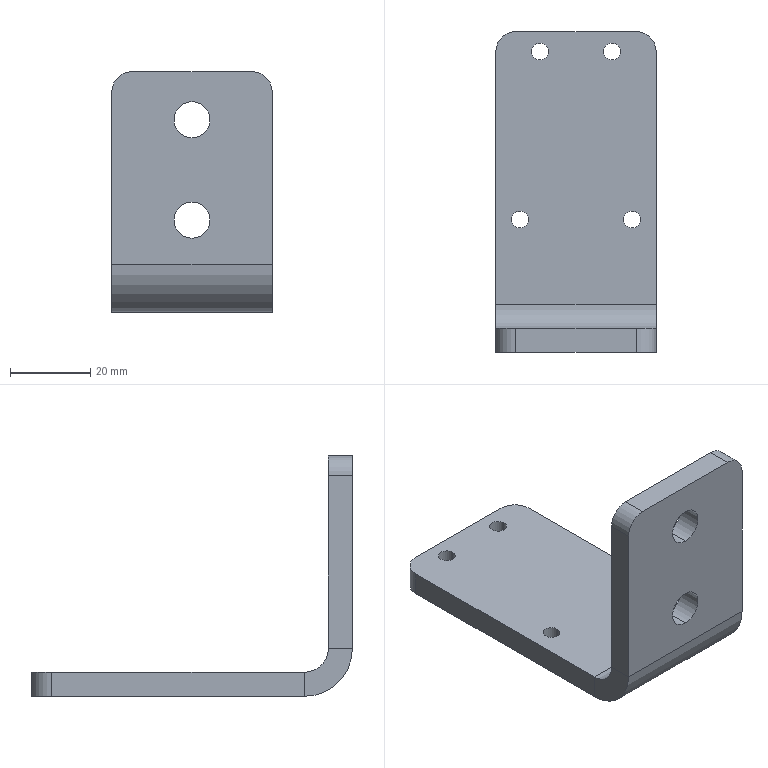Part | STEP file | 1 solid | 30 faces | box 40 x 80 x 60 mm | volume 30008 mm3 | cylinder 18 | plane 12 | commonest cylinder face diameters 4.2 x8 9 x4 10 x4 12 x1 24 x1